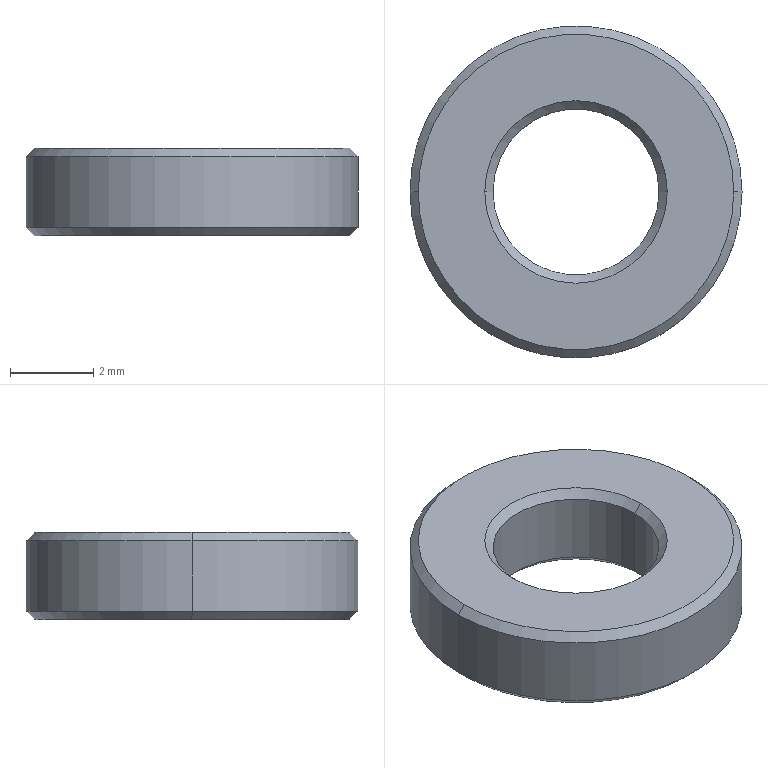Part | NX | features BREP 1 | 1 solid | 14 faces | box 8 x 8 x 2.1 mm | volume 77.66 mm3 | cone 8 | cylinder 4 | plane 2 | commonest cylinder face diameters 4 x2 8 x2
STEP:
#1=CARTESIAN_POINT('',(3.8,0.,1.05));
#2=VERTEX_POINT('',#1);
#3=CARTESIAN_POINT('',(4.,0.,0.85));
#4=VERTEX_POINT('',#3);
#5=CARTESIAN_POINT('',(3.8,0.,1.05));
#6=DIRECTION('',(0.7071,0.,-0.7071));
#7=VECTOR('',#6,1000.);
#8=LINE('',#5,#7);
#9=EDGE_CURVE('',#2,#4,#8,.T.);
#10=ORIENTED_EDGE('',*,*,#9,.F.);
#11=CARTESIAN_POINT('',(-3.8,0.,1.05));
#12=VERTEX_POINT('',#11);
#13=CARTESIAN_POINT('',(0.,0.,1.05));
#14=DIRECTION('',(0.,0.,1.));
#15=DIRECTION('',(1.,0.,0.));
#16=AXIS2_PLACEMENT_3D('',#13,#14,#15);
#17=CIRCLE('',#16,3.8);
#18=EDGE_CURVE('',#12,#2,#17,.T.);
#19=ORIENTED_EDGE('',*,*,#18,.F.);
#20=CARTESIAN_POINT('',(-4.,0.,0.85));
#21=VERTEX_POINT('',#20);
#22=CARTESIAN_POINT('',(-3.8,0.,1.05));
#23=DIRECTION('',(-0.7071,0.,-0.7071));
#24=VECTOR('',#23,1000.);
#25=LINE('',#22,#24);
#26=EDGE_CURVE('',#12,#21,#25,.T.);
#27=ORIENTED_EDGE('',*,*,#26,.T.);
#28=CARTESIAN_POINT('',(0.,0.,0.85));
#29=DIRECTION('',(0.,0.,-1.));
#30=DIRECTION('',(1.,0.,0.));
#31=AXIS2_PLACEMENT_3D('',#28,#29,#30);
#32=CIRCLE('',#31,4.);
#33=EDGE_CURVE('',#4,#21,#32,.T.);
#34=ORIENTED_EDGE('',*,*,#33,.F.);
#35=EDGE_LOOP('',(#10,#19,#27,#34));
#36=FACE_BOUND('',#35,.T.);
#37=CARTESIAN_POINT('',(0.,0.,1.05));
#38=DIRECTION('',(0.,0.,-1.));
#39=DIRECTION('',(-1.,0.,0.));
#40=AXIS2_PLACEMENT_3D('',#37,#38,#39);
#41=CONICAL_SURFACE('',#40,3.8,0.7854);
#42=ADVANCED_FACE('',(#36),#41,.T.);
#43=CARTESIAN_POINT('',(-4.,0.,-0.85));
#44=VERTEX_POINT('',#43);
#45=CARTESIAN_POINT('',(-3.8,0.,-1.05));
#46=VERTEX_POINT('',#45);
#47=CARTESIAN_POINT('',(-4.,0.,-0.85));
#48=DIRECTION('',(-0.7071,0.,0.7071));
#49=VECTOR('',#48,1000.);
#50=LINE('',#47,#49);
#51=EDGE_CURVE('',#44,#46,#50,.F.);
#52=ORIENTED_EDGE('',*,*,#51,.T.);
#53=CARTESIAN_POINT('',(3.8,0.,-1.05));
#54=VERTEX_POINT('',#53);
#55=CARTESIAN_POINT('',(0.,0.,-1.05));
#56=DIRECTION('',(0.,0.,-1.));
#57=DIRECTION('',(1.,0.,0.));
#58=AXIS2_PLACEMENT_3D('',#55,#56,#57);
#59=CIRCLE('',#58,3.8);
#60=EDGE_CURVE('',#54,#46,#59,.T.);
#61=ORIENTED_EDGE('',*,*,#60,.F.);
#62=CARTESIAN_POINT('',(4.,0.,-0.85));
#63=VERTEX_POINT('',#62);
#64=CARTESIAN_POINT('',(4.,0.,-0.85));
#65=DIRECTION('',(0.7071,0.,0.7071));
#66=VECTOR('',#65,1000.);
#67=LINE('',#64,#66);
#68=EDGE_CURVE('',#63,#54,#67,.F.);
#69=ORIENTED_EDGE('',*,*,#68,.F.);
#70=CARTESIAN_POINT('',(0.,0.,-0.85));
#71=DIRECTION('',(0.,0.,1.));
#72=DIRECTION('',(1.,0.,0.));
#73=AXIS2_PLACEMENT_3D('',#70,#71,#72);
#74=CIRCLE('',#73,4.);
#75=EDGE_CURVE('',#44,#63,#74,.T.);
#76=ORIENTED_EDGE('',*,*,#75,.F.);
#77=EDGE_LOOP('',(#52,#61,#69,#76));
#78=FACE_BOUND('',#77,.T.);
#79=CARTESIAN_POINT('',(0.,0.,-0.85));
#80=DIRECTION('',(0.,0.,1.));
#81=DIRECTION('',(1.,0.,0.));
#82=AXIS2_PLACEMENT_3D('',#79,#80,#81);
#83=CONICAL_SURFACE('',#82,4.,0.7854);
#84=ADVANCED_FACE('',(#78),#83,.T.);
#85=CARTESIAN_POINT('',(-2.2,0.,1.05));
#86=VERTEX_POINT('',#85);
#87=CARTESIAN_POINT('',(-2.,0.,0.85));
#88=VERTEX_POINT('',#87);
#89=CARTESIAN_POINT('',(-2.,0.,0.85));
#90=DIRECTION('',(-0.7071,0.,0.7071));
#91=VECTOR('',#90,1000.);
#92=LINE('',#89,#91);
#93=EDGE_CURVE('',#86,#88,#92,.F.);
#94=ORIENTED_EDGE('',*,*,#93,.T.);
#95=CARTESIAN_POINT('',(2.,0.,0.85));
#96=VERTEX_POINT('',#95);
#97=CARTESIAN_POINT('',(0.,0.,0.85));
#98=DIRECTION('',(0.,0.,1.));
#99=DIRECTION('',(1.,0.,0.));
#100=AXIS2_PLACEMENT_3D('',#97,#98,#99);
#101=CIRCLE('',#100,2.);
#102=EDGE_CURVE('',#96,#88,#101,.T.);
#103=ORIENTED_EDGE('',*,*,#102,.F.);
#104=CARTESIAN_POINT('',(2.2,0.,1.05));
#105=VERTEX_POINT('',#104);
#106=CARTESIAN_POINT('',(2.,0.,0.85));
#107=DIRECTION('',(0.7071,0.,0.7071));
#108=VECTOR('',#107,1000.);
#109=LINE('',#106,#108);
#110=EDGE_CURVE('',#105,#96,#109,.F.);
#111=ORIENTED_EDGE('',*,*,#110,.F.);
#112=CARTESIAN_POINT('',(0.,0.,1.05));
#113=DIRECTION('',(0.,0.,-1.));
#114=DIRECTION('',(1.,0.,0.));
#115=AXIS2_PLACEMENT_3D('',#112,#113,#114);
#116=CIRCLE('',#115,2.2);
#117=EDGE_CURVE('',#86,#105,#116,.T.);
#118=ORIENTED_EDGE('',*,*,#117,.F.);
#119=EDGE_LOOP('',(#94,#103,#111,#118));
#120=FACE_BOUND('',#119,.T.);
#121=CARTESIAN_POINT('',(0.,0.,0.85));
#122=DIRECTION('',(0.,0.,1.));
#123=DIRECTION('',(1.,0.,0.));
#124=AXIS2_PLACEMENT_3D('',#121,#122,#123);
#125=CONICAL_SURFACE('',#124,2.,0.7854);
#126=ADVANCED_FACE('',(#120),#125,.F.);
#127=CARTESIAN_POINT('',(2.,0.,-0.85));
#128=VERTEX_POINT('',#127);
#129=CARTESIAN_POINT('',(2.2,0.,-1.05));
#130=VERTEX_POINT('',#129);
#131=CARTESIAN_POINT('',(2.2,0.,-1.05));
#132=DIRECTION('',(0.7071,0.,-0.7071));
#133=VECTOR('',#132,1000.);
#134=LINE('',#131,#133);
#135=EDGE_CURVE('',#128,#130,#134,.T.);
#136=ORIENTED_EDGE('',*,*,#135,.F.);
#137=CARTESIAN_POINT('',(-2.,0.,-0.85));
#138=VERTEX_POINT('',#137);
#139=CARTESIAN_POINT('',(0.,0.,-0.85));
#140=DIRECTION('',(0.,0.,-1.));
#141=DIRECTION('',(1.,0.,0.));
#142=AXIS2_PLACEMENT_3D('',#139,#140,#141);
#143=CIRCLE('',#142,2.);
#144=EDGE_CURVE('',#138,#128,#143,.T.);
#145=ORIENTED_EDGE('',*,*,#144,.F.);
#146=CARTESIAN_POINT('',(-2.2,0.,-1.05));
#147=VERTEX_POINT('',#146);
#148=CARTESIAN_POINT('',(-2.2,0.,-1.05));
#149=DIRECTION('',(-0.7071,0.,-0.7071));
#150=VECTOR('',#149,1000.);
#151=LINE('',#148,#150);
#152=EDGE_CURVE('',#138,#147,#151,.T.);
#153=ORIENTED_EDGE('',*,*,#152,.T.);
#154=CARTESIAN_POINT('',(0.,0.,-1.05));
#155=DIRECTION('',(0.,0.,1.));
#156=DIRECTION('',(1.,0.,0.));
#157=AXIS2_PLACEMENT_3D('',#154,#155,#156);
#158=CIRCLE('',#157,2.2);
#159=EDGE_CURVE('',#130,#147,#158,.T.);
#160=ORIENTED_EDGE('',*,*,#159,.F.);
#161=EDGE_LOOP('',(#136,#145,#153,#160));
#162=FACE_BOUND('',#161,.T.);
#163=CARTESIAN_POINT('',(0.,0.,-1.05));
#164=DIRECTION('',(0.,0.,-1.));
#165=DIRECTION('',(-1.,0.,0.));
#166=AXIS2_PLACEMENT_3D('',#163,#164,#165);
#167=CONICAL_SURFACE('',#166,2.2,0.7854);
#168=ADVANCED_FACE('',(#162),#167,.F.);
#169=CARTESIAN_POINT('',(2.,0.,1.05));
#170=DIRECTION('',(0.,0.,-1.));
#171=VECTOR('',#170,1000.);
#172=LINE('',#169,#171);
#173=EDGE_CURVE('',#96,#128,#172,.T.);
#174=ORIENTED_EDGE('',*,*,#173,.F.);
#175=ORIENTED_EDGE('',*,*,#102,.T.);
#176=CARTESIAN_POINT('',(-2.,0.,1.05));
#177=DIRECTION('',(0.,0.,-1.));
#178=VECTOR('',#177,1000.);
#179=LINE('',#176,#178);
#180=EDGE_CURVE('',#88,#138,#179,.T.);
#181=ORIENTED_EDGE('',*,*,#180,.T.);
#182=ORIENTED_EDGE('',*,*,#144,.T.);
#183=EDGE_LOOP('',(#174,#175,#181,#182));
#184=FACE_BOUND('',#183,.T.);
#185=CARTESIAN_POINT('',(0.,0.,1.05));
#186=DIRECTION('',(0.,0.,-1.));
#187=DIRECTION('',(-1.,0.,0.));
#188=AXIS2_PLACEMENT_3D('',#185,#186,#187);
#189=CYLINDRICAL_SURFACE('',#188,2.);
#190=ADVANCED_FACE('',(#184),#189,.F.);
#191=CARTESIAN_POINT('',(4.,0.,1.05));
#192=DIRECTION('',(0.,0.,-1.));
#193=VECTOR('',#192,1000.);
#194=LINE('',#191,#193);
#195=EDGE_CURVE('',#4,#63,#194,.T.);
#196=ORIENTED_EDGE('',*,*,#195,.F.);
#197=ORIENTED_EDGE('',*,*,#33,.T.);
#198=CARTESIAN_POINT('',(-4.,0.,1.05));
#199=DIRECTION('',(0.,0.,-1.));
#200=VECTOR('',#199,1000.);
#201=LINE('',#198,#200);
#202=EDGE_CURVE('',#21,#44,#201,.T.);
#203=ORIENTED_EDGE('',*,*,#202,.T.);
#204=ORIENTED_EDGE('',*,*,#75,.T.);
#205=EDGE_LOOP('',(#196,#197,#203,#204));
#206=FACE_BOUND('',#205,.T.);
#207=CARTESIAN_POINT('',(0.,0.,1.05));
#208=DIRECTION('',(0.,0.,-1.));
#209=DIRECTION('',(-1.,0.,0.));
#210=AXIS2_PLACEMENT_3D('',#207,#208,#209);
#211=CYLINDRICAL_SURFACE('',#210,4.);
#212=ADVANCED_FACE('',(#206),#211,.T.);
#213=ORIENTED_EDGE('',*,*,#60,.T.);
#214=CARTESIAN_POINT('',(0.,0.,-1.05));
#215=DIRECTION('',(0.,0.,-1.));
#216=DIRECTION('',(1.,0.,0.));
#217=AXIS2_PLACEMENT_3D('',#214,#215,#216);
#218=CIRCLE('',#217,3.8);
#219=EDGE_CURVE('',#46,#54,#218,.T.);
#220=ORIENTED_EDGE('',*,*,#219,.T.);
#221=EDGE_LOOP('',(#213,#220));
#222=FACE_BOUND('',#221,.T.);
#223=CARTESIAN_POINT('',(0.,0.,-1.05));
#224=DIRECTION('',(0.,0.,1.));
#225=DIRECTION('',(1.,0.,0.));
#226=AXIS2_PLACEMENT_3D('',#223,#224,#225);
#227=CIRCLE('',#226,2.2);
#228=EDGE_CURVE('',#147,#130,#227,.T.);
#229=ORIENTED_EDGE('',*,*,#228,.T.);
#230=ORIENTED_EDGE('',*,*,#159,.T.);
#231=EDGE_LOOP('',(#229,#230));
#232=FACE_BOUND('',#231,.T.);
#233=CARTESIAN_POINT('',(0.,0.,-1.05));
#234=DIRECTION('',(0.,0.,1.));
#235=DIRECTION('',(1.,0.,0.));
#236=AXIS2_PLACEMENT_3D('',#233,#234,#235);
#237=PLANE('',#236);
#238=ADVANCED_FACE('',(#222,#232),#237,.F.);
#239=ORIENTED_EDGE('',*,*,#18,.T.);
#240=CARTESIAN_POINT('',(0.,0.,1.05));
#241=DIRECTION('',(0.,0.,1.));
#242=DIRECTION('',(1.,0.,0.));
#243=AXIS2_PLACEMENT_3D('',#240,#241,#242);
#244=CIRCLE('',#243,3.8);
#245=EDGE_CURVE('',#2,#12,#244,.T.);
#246=ORIENTED_EDGE('',*,*,#245,.T.);
#247=EDGE_LOOP('',(#239,#246));
#248=FACE_BOUND('',#247,.T.);
#249=CARTESIAN_POINT('',(0.,0.,1.05));
#250=DIRECTION('',(0.,0.,-1.));
#251=DIRECTION('',(1.,0.,0.));
#252=AXIS2_PLACEMENT_3D('',#249,#250,#251);
#253=CIRCLE('',#252,2.2);
#254=EDGE_CURVE('',#105,#86,#253,.T.);
#255=ORIENTED_EDGE('',*,*,#254,.T.);
#256=ORIENTED_EDGE('',*,*,#117,.T.);
#257=EDGE_LOOP('',(#255,#256));
#258=FACE_BOUND('',#257,.T.);
#259=CARTESIAN_POINT('',(0.,0.,1.05));
#260=DIRECTION('',(0.,0.,1.));
#261=DIRECTION('',(1.,0.,0.));
#262=AXIS2_PLACEMENT_3D('',#259,#260,#261);
#263=PLANE('',#262);
#264=ADVANCED_FACE('',(#248,#258),#263,.T.);
#265=CARTESIAN_POINT('',(0.,0.,0.85));
#266=DIRECTION('',(0.,0.,-1.));
#267=DIRECTION('',(1.,0.,0.));
#268=AXIS2_PLACEMENT_3D('',#265,#266,#267);
#269=CIRCLE('',#268,4.);
#270=EDGE_CURVE('',#21,#4,#269,.T.);
#271=ORIENTED_EDGE('',*,*,#270,.T.);
#272=ORIENTED_EDGE('',*,*,#195,.T.);
#273=CARTESIAN_POINT('',(0.,0.,-0.85));
#274=DIRECTION('',(0.,0.,1.));
#275=DIRECTION('',(1.,0.,0.));
#276=AXIS2_PLACEMENT_3D('',#273,#274,#275);
#277=CIRCLE('',#276,4.);
#278=EDGE_CURVE('',#63,#44,#277,.T.);
#279=ORIENTED_EDGE('',*,*,#278,.T.);
#280=ORIENTED_EDGE('',*,*,#202,.F.);
#281=EDGE_LOOP('',(#271,#272,#279,#280));
#282=FACE_BOUND('',#281,.T.);
#283=CARTESIAN_POINT('',(0.,0.,1.05));
#284=DIRECTION('',(0.,0.,-1.));
#285=DIRECTION('',(-1.,0.,0.));
#286=AXIS2_PLACEMENT_3D('',#283,#284,#285);
#287=CYLINDRICAL_SURFACE('',#286,4.);
#288=ADVANCED_FACE('',(#282),#287,.T.);
#289=CARTESIAN_POINT('',(0.,0.,0.85));
#290=DIRECTION('',(0.,0.,1.));
#291=DIRECTION('',(1.,0.,0.));
#292=AXIS2_PLACEMENT_3D('',#289,#290,#291);
#293=CIRCLE('',#292,2.);
#294=EDGE_CURVE('',#88,#96,#293,.T.);
#295=ORIENTED_EDGE('',*,*,#294,.T.);
#296=ORIENTED_EDGE('',*,*,#173,.T.);
#297=CARTESIAN_POINT('',(0.,0.,-0.85));
#298=DIRECTION('',(0.,0.,-1.));
#299=DIRECTION('',(1.,0.,0.));
#300=AXIS2_PLACEMENT_3D('',#297,#298,#299);
#301=CIRCLE('',#300,2.);
#302=EDGE_CURVE('',#128,#138,#301,.T.);
#303=ORIENTED_EDGE('',*,*,#302,.T.);
#304=ORIENTED_EDGE('',*,*,#180,.F.);
#305=EDGE_LOOP('',(#295,#296,#303,#304));
#306=FACE_BOUND('',#305,.T.);
#307=CARTESIAN_POINT('',(0.,0.,1.05));
#308=DIRECTION('',(0.,0.,-1.));
#309=DIRECTION('',(-1.,0.,0.));
#310=AXIS2_PLACEMENT_3D('',#307,#308,#309);
#311=CYLINDRICAL_SURFACE('',#310,2.);
#312=ADVANCED_FACE('',(#306),#311,.F.);
#313=ORIENTED_EDGE('',*,*,#302,.F.);
#314=ORIENTED_EDGE('',*,*,#135,.T.);
#315=ORIENTED_EDGE('',*,*,#228,.F.);
#316=ORIENTED_EDGE('',*,*,#152,.F.);
#317=EDGE_LOOP('',(#313,#314,#315,#316));
#318=FACE_BOUND('',#317,.T.);
#319=CARTESIAN_POINT('',(0.,0.,-1.05));
#320=DIRECTION('',(0.,0.,-1.));
#321=DIRECTION('',(-1.,0.,0.));
#322=AXIS2_PLACEMENT_3D('',#319,#320,#321);
#323=CONICAL_SURFACE('',#322,2.2,0.7854);
#324=ADVANCED_FACE('',(#318),#323,.F.);
#325=ORIENTED_EDGE('',*,*,#294,.F.);
#326=ORIENTED_EDGE('',*,*,#93,.F.);
#327=ORIENTED_EDGE('',*,*,#254,.F.);
#328=ORIENTED_EDGE('',*,*,#110,.T.);
#329=EDGE_LOOP('',(#325,#326,#327,#328));
#330=FACE_BOUND('',#329,.T.);
#331=CARTESIAN_POINT('',(0.,0.,0.85));
#332=DIRECTION('',(0.,0.,1.));
#333=DIRECTION('',(1.,0.,0.));
#334=AXIS2_PLACEMENT_3D('',#331,#332,#333);
#335=CONICAL_SURFACE('',#334,2.,0.7854);
#336=ADVANCED_FACE('',(#330),#335,.F.);
#337=ORIENTED_EDGE('',*,*,#219,.F.);
#338=ORIENTED_EDGE('',*,*,#51,.F.);
#339=ORIENTED_EDGE('',*,*,#278,.F.);
#340=ORIENTED_EDGE('',*,*,#68,.T.);
#341=EDGE_LOOP('',(#337,#338,#339,#340));
#342=FACE_BOUND('',#341,.T.);
#343=CARTESIAN_POINT('',(0.,0.,-0.85));
#344=DIRECTION('',(0.,0.,1.));
#345=DIRECTION('',(1.,0.,0.));
#346=AXIS2_PLACEMENT_3D('',#343,#344,#345);
#347=CONICAL_SURFACE('',#346,4.,0.7854);
#348=ADVANCED_FACE('',(#342),#347,.T.);
#349=ORIENTED_EDGE('',*,*,#245,.F.);
#350=ORIENTED_EDGE('',*,*,#9,.T.);
#351=ORIENTED_EDGE('',*,*,#270,.F.);
#352=ORIENTED_EDGE('',*,*,#26,.F.);
#353=EDGE_LOOP('',(#349,#350,#351,#352));
#354=FACE_BOUND('',#353,.T.);
#355=CARTESIAN_POINT('',(0.,0.,1.05));
#356=DIRECTION('',(0.,0.,-1.));
#357=DIRECTION('',(-1.,0.,0.));
#358=AXIS2_PLACEMENT_3D('',#355,#356,#357);
#359=CONICAL_SURFACE('',#358,3.8,0.7854);
#360=ADVANCED_FACE('',(#354),#359,.T.);
#361=CLOSED_SHELL('',(#42,#84,#126,#168,#190,#212,#238,#264,#288,#312,#324,#336,#348,#360));
#362=MANIFOLD_SOLID_BREP('',#361);
#363=(LENGTH_UNIT()NAMED_UNIT(*)SI_UNIT(.MILLI.,.METRE.));
#364=UNCERTAINTY_MEASURE_WITH_UNIT(LENGTH_MEASURE(0.00001),#363,'','');
#365=(NAMED_UNIT(*)PLANE_ANGLE_UNIT()SI_UNIT($,.RADIAN.));
#366=(NAMED_UNIT(*)SI_UNIT($,.STERADIAN.)SOLID_ANGLE_UNIT());
#367=(GEOMETRIC_REPRESENTATION_CONTEXT(3)GLOBAL_UNCERTAINTY_ASSIGNED_CONTEXT((#364))GLOBAL_UNIT_ASSIGNED_CONTEXT((#363,#365,#366))REPRESENTATION_CONTEXT('',''));
#368=ADVANCED_BREP_SHAPE_REPRESENTATION('',(#362),#367);